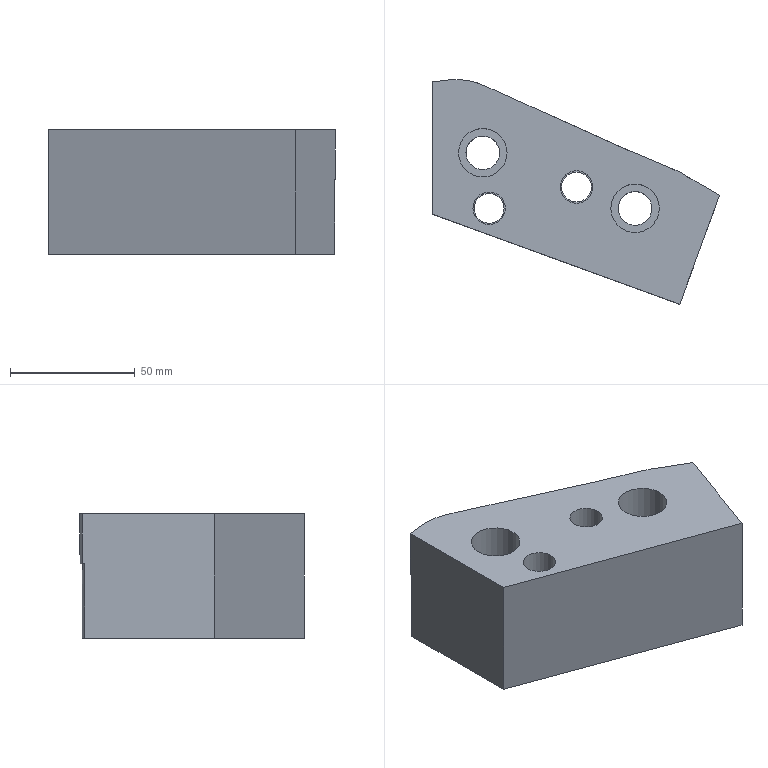Part | NX | features solid 2 | 1 solid | 23 faces | box 115.07 x 90.062 x 50 mm | volume 264486 mm3 | plane 13 | cylinder 8 | spline 2 | commonest cylinder face diameters 12 x2 13 x2 13.5 x2 19.5 x2
STEP:
#1=CARTESIAN_POINT('',(409.722,86.331,-20.));
#2=VERTEX_POINT('',#1);
#3=CARTESIAN_POINT('',(396.631,93.889,-20.));
#4=VERTEX_POINT('',#3);
#5=CARTESIAN_POINT('',(49.747,294.163,-20.));
#6=DIRECTION('',(0.866,-0.5,0.));
#7=VECTOR('',#6,1000.);
#8=LINE('',#5,#7);
#9=EDGE_CURVE('',#2,#4,#8,.F.);
#10=ORIENTED_EDGE('',*,*,#9,.T.);
#11=CARTESIAN_POINT('',(295.,131.707,-20.));
#12=VERTEX_POINT('',#11);
#13=CARTESIAN_POINT('',(396.631,93.889,-20.));
#14=CARTESIAN_POINT('',(395.875,94.532,-20.));
#15=CARTESIAN_POINT('',(393.947,95.547,-20.));
#16=CARTESIAN_POINT('',(390.75,97.031,-20.));
#17=CARTESIAN_POINT('',(387.669,98.355,-20.));
#18=CARTESIAN_POINT('',(383.326,99.967,-20.));
#19=CARTESIAN_POINT('',(377.97,102.219,-20.));
#20=CARTESIAN_POINT('',(369.545,105.997,-20.));
#21=CARTESIAN_POINT('',(359.032,110.723,-20.));
#22=CARTESIAN_POINT('',(346.404,116.383,-20.));
#23=CARTESIAN_POINT('',(335.885,121.105,-20.));
#24=CARTESIAN_POINT('',(327.471,124.89,-20.));
#25=CARTESIAN_POINT('',(322.219,127.254,-20.));
#26=CARTESIAN_POINT('',(318.003,129.177,-20.));
#27=CARTESIAN_POINT('',(314.891,130.622,-20.));
#28=CARTESIAN_POINT('',(311.756,131.732,-20.));
#29=CARTESIAN_POINT('',(307.396,132.672,-20.));
#30=CARTESIAN_POINT('',(301.819,132.728,-20.));
#31=CARTESIAN_POINT('',(297.285,132.035,-20.));
#32=CARTESIAN_POINT('',(295.,131.707,-20.));
#33=B_SPLINE_CURVE_WITH_KNOTS('',3,(#13,#14,#15,#16,#17,#18,#19,#20,#21,#22,#23,#24,#25,#26,#27,#28,#29,#30,#31,#32),.UNSPECIFIED.,.F.,.F.,(4,1,1,1,1,1,1,1,1,1,1,1,1,1,1,1,1,4),(0.7727,0.7742,0.7756,0.7771,0.7786,0.7816,0.7845,0.7904,0.7964,0.8023,0.8052,0.8082,0.8097,0.8112,0.8126,0.8141,0.8171,0.82),.UNSPECIFIED.);
#34=EDGE_CURVE('',#4,#12,#33,.T.);
#35=ORIENTED_EDGE('',*,*,#34,.T.);
#36=CARTESIAN_POINT('',(295.,132.717,-20.));
#37=VERTEX_POINT('',#36);
#38=CARTESIAN_POINT('',(295.,32.206,-20.));
#39=DIRECTION('',(0.,1.,0.));
#40=VECTOR('',#39,1000.);
#41=LINE('',#38,#40);
#42=EDGE_CURVE('',#12,#37,#41,.T.);
#43=ORIENTED_EDGE('',*,*,#42,.T.);
#44=CARTESIAN_POINT('',(397.207,94.712,-20.));
#45=VERTEX_POINT('',#44);
#46=CARTESIAN_POINT('',(-190.231,-121.49,-20.));
#47=CARTESIAN_POINT('',(-188.654,-121.152,-20.));
#48=CARTESIAN_POINT('',(-185.47,-120.627,-20.));
#49=CARTESIAN_POINT('',(-180.656,-120.141,-20.));
#50=CARTESIAN_POINT('',(-175.882,-119.326,-20.));
#51=CARTESIAN_POINT('',(-169.679,-117.528,-20.));
#52=CARTESIAN_POINT('',(-162.185,-114.539,-20.));
#53=CARTESIAN_POINT('',(-153.086,-111.254,-20.));
#54=CARTESIAN_POINT('',(-144.031,-107.845,-20.));
#55=CARTESIAN_POINT('',(-136.465,-105.061,-20.));
#56=CARTESIAN_POINT('',(-130.418,-102.814,-20.));
#57=CARTESIAN_POINT('',(-125.812,-101.329,-20.));
#58=CARTESIAN_POINT('',(-121.306,-99.566,-20.));
#59=CARTESIAN_POINT('',(-116.876,-97.626,-20.));
#60=CARTESIAN_POINT('',(-112.335,-95.923,-20.));
#61=CARTESIAN_POINT('',(-107.564,-95.05,-20.));
#62=CARTESIAN_POINT('',(-102.756,-94.525,-20.));
#63=CARTESIAN_POINT('',(-96.349,-93.771,-20.));
#64=CARTESIAN_POINT('',(-89.902,-93.468,-20.));
#65=CARTESIAN_POINT('',(-83.452,-93.448,-20.));
#66=CARTESIAN_POINT('',(-77.002,-93.469,-20.));
#67=CARTESIAN_POINT('',(-68.939,-93.411,-20.));
#68=CARTESIAN_POINT('',(-56.04,-93.3,-20.));
#69=CARTESIAN_POINT('',(-33.465,-93.184,-20.));
#70=CARTESIAN_POINT('',(-7.666,-93.074,-20.));
#71=CARTESIAN_POINT('',(14.907,-92.653,-20.));
#72=CARTESIAN_POINT('',(27.794,-92.068,-20.));
#73=CARTESIAN_POINT('',(40.668,-91.245,-20.));
#74=CARTESIAN_POINT('',(51.917,-90.291,-20.));
#75=CARTESIAN_POINT('',(61.528,-89.174,-20.));
#76=CARTESIAN_POINT('',(67.939,-88.466,-20.));
#77=CARTESIAN_POINT('',(79.125,-86.95,-20.));
#78=CARTESIAN_POINT('',(95.161,-85.253,-20.));
#79=CARTESIAN_POINT('',(114.404,-83.21,-20.));
#80=CARTESIAN_POINT('',(133.568,-80.524,-20.));
#81=CARTESIAN_POINT('',(152.734,-77.861,-20.));
#82=CARTESIAN_POINT('',(171.916,-75.326,-20.));
#83=CARTESIAN_POINT('',(191.055,-72.413,-20.));
#84=CARTESIAN_POINT('',(207.17,-71.468,-20.));
#85=CARTESIAN_POINT('',(219.951,-69.697,-20.));
#86=CARTESIAN_POINT('',(232.724,-67.899,-20.));
#87=CARTESIAN_POINT('',(248.708,-65.766,-20.));
#88=CARTESIAN_POINT('',(267.87,-63.074,-20.));
#89=CARTESIAN_POINT('',(287.038,-60.44,-20.));
#90=CARTESIAN_POINT('',(301.448,-58.682,-20.));
#91=CARTESIAN_POINT('',(310.976,-56.987,-20.));
#92=CARTESIAN_POINT('',(314.916,-56.135,-20.));
#93=CARTESIAN_POINT('',(318.052,-55.382,-20.));
#94=CARTESIAN_POINT('',(320.39,-54.76,-20.));
#95=CARTESIAN_POINT('',(322.686,-53.981,-20.));
#96=CARTESIAN_POINT('',(325.595,-52.578,-20.));
#97=CARTESIAN_POINT('',(328.769,-50.098,-20.));
#98=CARTESIAN_POINT('',(332.247,-46.69,-20.));
#99=CARTESIAN_POINT('',(335.795,-43.406,-20.));
#100=CARTESIAN_POINT('',(343.661,-37.758,-20.));
#101=CARTESIAN_POINT('',(355.164,-28.914,-20.));
#102=CARTESIAN_POINT('',(370.422,-17.018,-20.));
#103=CARTESIAN_POINT('',(383.264,-7.249,-20.));
#104=CARTESIAN_POINT('',(392.416,-0.6713,-20.));
#105=CARTESIAN_POINT('',(396.953,2.733,-20.));
#106=CARTESIAN_POINT('',(398.886,5.372,-20.));
#107=CARTESIAN_POINT('',(399.725,7.654,-20.));
#108=CARTESIAN_POINT('',(399.76,10.078,-20.));
#109=CARTESIAN_POINT('',(399.483,13.317,-20.));
#110=CARTESIAN_POINT('',(399.712,17.34,-20.));
#111=CARTESIAN_POINT('',(399.612,22.179,-20.));
#112=CARTESIAN_POINT('',(399.633,31.854,-20.));
#113=CARTESIAN_POINT('',(399.593,46.366,-20.));
#114=CARTESIAN_POINT('',(399.637,62.491,-20.));
#115=CARTESIAN_POINT('',(399.588,73.779,-20.));
#116=CARTESIAN_POINT('',(399.652,79.422,-20.));
#117=CARTESIAN_POINT('',(399.59,82.647,-20.));
#118=CARTESIAN_POINT('',(399.564,85.065,-20.));
#119=CARTESIAN_POINT('',(399.725,87.486,-20.));
#120=CARTESIAN_POINT('',(399.756,89.902,-20.));
#121=CARTESIAN_POINT('',(399.247,92.301,-20.));
#122=CARTESIAN_POINT('',(397.362,95.008,-20.));
#123=CARTESIAN_POINT('',(393.635,96.774,-20.));
#124=CARTESIAN_POINT('',(389.279,98.826,-20.));
#125=CARTESIAN_POINT('',(384.732,100.498,-20.));
#126=CARTESIAN_POINT('',(378.765,102.95,-20.));
#127=CARTESIAN_POINT('',(362.589,110.229,-20.));
#128=CARTESIAN_POINT('',(344.928,118.135,-20.));
#129=CARTESIAN_POINT('',(327.281,126.072,-20.));
#130=CARTESIAN_POINT('',(319.932,129.381,-20.));
#131=CARTESIAN_POINT('',(314.075,132.102,-20.));
#132=CARTESIAN_POINT('',(309.387,133.376,-20.));
#133=CARTESIAN_POINT('',(304.547,133.785,-20.));
#134=CARTESIAN_POINT('',(299.716,133.401,-20.));
#135=CARTESIAN_POINT('',(294.929,132.704,-20.));
#136=CARTESIAN_POINT('',(288.543,131.8,-20.));
#137=CARTESIAN_POINT('',(277.364,130.241,-20.));
#138=CARTESIAN_POINT('',(242.2,125.552,-20.));
#139=CARTESIAN_POINT('',(184.637,118.048,-20.));
#140=CARTESIAN_POINT('',(120.701,109.541,-20.));
#141=CARTESIAN_POINT('',(69.531,102.902,-20.));
#142=CARTESIAN_POINT('',(40.777,98.94,-20.));
#143=CARTESIAN_POINT('',(21.566,96.615,-20.));
#144=CARTESIAN_POINT('',(8.743,95.212,-20.));
#145=CARTESIAN_POINT('',(-7.301,93.575,-20.));
#146=CARTESIAN_POINT('',(-26.625,92.505,-20.));
#147=CARTESIAN_POINT('',(-45.971,92.017,-20.));
#148=CARTESIAN_POINT('',(-62.09,91.675,-20.));
#149=CARTESIAN_POINT('',(-74.987,91.256,-20.));
#150=CARTESIAN_POINT('',(-84.664,91.165,-20.));
#151=CARTESIAN_POINT('',(-94.319,91.781,-20.));
#152=CARTESIAN_POINT('',(-103.929,92.966,-20.));
#153=CARTESIAN_POINT('',(-113.495,94.403,-20.));
#154=CARTESIAN_POINT('',(-119.856,95.492,-20.));
#155=CARTESIAN_POINT('',(-122.997,96.222,-20.));
#156=B_SPLINE_CURVE_WITH_KNOTS('',3,(#46,#47,#48,#49,#50,#51,#52,#53,#54,#55,#56,#57,#58,#59,#60,#61,#62,#63,#64,#65,#66,#67,#68,#69,#70,#71,#72,#73,#74,#75,#76,#77,#78,#79,#80,#81,#82,#83,#84,#85,#86,#87,#88,#89,#90,#91,#92,#93,#94,#95,#96,#97,#98,#99,#100,#101,#102,#103,#104,#105,#106,#107,#108,#109,#110,#111,#112,#113,#114,#115,#116,#117,#118,#119,#120,#121,#122,#123,#124,#125,#126,#127,#128,#129,#130,#131,#132,#133,#134,#135,#136,#137,#138,#139,#140,#141,#142,#143,#144,#145,#146,#147,#148,#149,#150,#151,#152,#153,#154,#155),.UNSPECIFIED.,.F.,.F.,(4,1,1,1,1,1,1,1,1,1,1,1,1,1,1,1,1,1,1,1,1,1,1,1,1,1,1,1,1,1,1,1,1,1,1,1,1,1,1,1,1,1,1,1,1,1,1,1,1,1,1,1,1,1,1,1,1,1,1,1,1,1,1,1,1,1,1,1,1,1,1,1,1,1,1,1,1,1,1,1,1,1,1,1,1,1,1,1,1,1,1,1,1,1,1,1,1,1,1,1,1,1,1,1,1,1,1,4),(0.4704,0.4724,0.4745,0.4766,0.4786,0.4828,0.4869,0.491,0.4952,0.4972,0.4993,0.5014,0.5035,0.5055,0.5076,0.5097,0.5117,0.5159,0.5179,0.52,0.5241,0.5283,0.5366,0.5531,0.5614,0.5655,0.5697,0.5779,0.58,0.5821,0.5862,0.5945,0.6028,0.611,0.6193,0.6276,0.6359,0.6441,0.6483,0.6524,0.6607,0.669,0.6772,0.6855,0.6876,0.6897,0.6907,0.6917,0.6928,0.6938,0.6959,0.6979,0.7,0.7021,0.7103,0.7186,0.7269,0.731,0.7331,0.7341,0.7352,0.7362,0.7372,0.7393,0.7414,0.7435,0.7517,0.76,0.7641,0.7662,0.7672,0.7683,0.7693,0.7703,0.7714,0.7724,0.7745,0.7766,0.7786,0.7807,0.7848,0.8014,0.8055,0.8097,0.8117,0.8138,0.8159,0.8179,0.82,0.8221,0.8262,0.8345,0.8676,0.9007,0.9172,0.9338,0.9379,0.9421,0.9503,0.9586,0.9669,0.9752,0.9793,0.9834,0.9876,0.9917,0.9959,1.),.UNSPECIFIED.);
#157=EDGE_CURVE('',#45,#37,#156,.T.);
#158=ORIENTED_EDGE('',*,*,#157,.F.);
#159=CARTESIAN_POINT('',(410.07,87.285,-20.));
#160=VERTEX_POINT('',#159);
#161=CARTESIAN_POINT('',(409.267,87.749,-20.));
#162=DIRECTION('',(-0.866,0.5,0.));
#163=VECTOR('',#162,1000.);
#164=LINE('',#161,#163);
#165=EDGE_CURVE('',#160,#45,#164,.T.);
#166=ORIENTED_EDGE('',*,*,#165,.F.);
#167=CARTESIAN_POINT('',(395.302,46.71,-20.));
#168=DIRECTION('',(-0.342,-0.9397,0.));
#169=VECTOR('',#168,1000.);
#170=LINE('',#167,#169);
#171=EDGE_CURVE('',#160,#2,#170,.T.);
#172=ORIENTED_EDGE('',*,*,#171,.T.);
#173=EDGE_LOOP('',(#10,#35,#43,#158,#166,#172));
#174=FACE_BOUND('',#173,.T.);
#175=CARTESIAN_POINT('',(-190.231,-121.49,-20.));
#176=DIRECTION('',(0.,0.,1.));
#177=DIRECTION('',(1.,0.,0.));
#178=AXIS2_PLACEMENT_3D('',#175,#176,#177);
#179=PLANE('',#178);
#180=ADVANCED_FACE('',(#174),#179,.F.);
#181=CARTESIAN_POINT('',(396.631,93.889,-50.));
#182=VERTEX_POINT('',#181);
#183=CARTESIAN_POINT('',(396.631,93.889,-35.));
#184=DIRECTION('',(0.,0.,-1.));
#185=VECTOR('',#184,1000.);
#186=LINE('',#183,#185);
#187=EDGE_CURVE('',#182,#4,#186,.F.);
#188=ORIENTED_EDGE('',*,*,#187,.F.);
#189=CARTESIAN_POINT('',(295.,131.707,-50.));
#190=VERTEX_POINT('',#189);
#191=CARTESIAN_POINT('',(295.,131.707,-50.));
#192=CARTESIAN_POINT('',(297.276,132.034,-50.));
#193=CARTESIAN_POINT('',(301.806,132.738,-50.));
#194=CARTESIAN_POINT('',(307.62,132.66,-50.));
#195=CARTESIAN_POINT('',(312.106,131.636,-50.));
#196=CARTESIAN_POINT('',(315.302,130.443,-50.));
#197=CARTESIAN_POINT('',(318.413,128.985,-50.));
#198=CARTESIAN_POINT('',(322.577,127.094,-50.));
#199=CARTESIAN_POINT('',(327.792,124.745,-50.));
#200=CARTESIAN_POINT('',(336.136,120.993,-50.));
#201=CARTESIAN_POINT('',(346.569,116.309,-50.));
#202=CARTESIAN_POINT('',(359.092,110.696,-50.));
#203=CARTESIAN_POINT('',(369.523,106.007,-50.));
#204=CARTESIAN_POINT('',(377.871,102.264,-50.));
#205=CARTESIAN_POINT('',(383.139,100.041,-50.));
#206=CARTESIAN_POINT('',(387.428,98.446,-50.));
#207=CARTESIAN_POINT('',(390.592,97.111,-50.));
#208=CARTESIAN_POINT('',(393.681,95.654,-50.));
#209=CARTESIAN_POINT('',(395.755,94.633,-50.));
#210=CARTESIAN_POINT('',(396.631,93.889,-50.));
#211=B_SPLINE_CURVE_WITH_KNOTS('',3,(#191,#192,#193,#194,#195,#196,#197,#198,#199,#200,#201,#202,#203,#204,#205,#206,#207,#208,#209,#210),.UNSPECIFIED.,.F.,.F.,(4,1,1,1,1,1,1,1,1,1,1,1,1,1,1,1,1,4),(0.,0.006873,0.01375,0.01718,0.02062,0.02406,0.02749,0.03437,0.04124,0.05499,0.06873,0.08248,0.08935,0.09623,0.09966,0.1031,0.1065,0.11),.UNSPECIFIED.);
#212=EDGE_CURVE('',#190,#182,#211,.T.);
#213=ORIENTED_EDGE('',*,*,#212,.F.);
#214=CARTESIAN_POINT('',(295.,131.707,-60.));
#215=DIRECTION('',(0.,0.,-1.));
#216=VECTOR('',#215,1000.);
#217=LINE('',#214,#216);
#218=EDGE_CURVE('',#190,#12,#217,.F.);
#219=ORIENTED_EDGE('',*,*,#218,.T.);
#220=ORIENTED_EDGE('',*,*,#34,.F.);
#221=EDGE_LOOP('',(#188,#213,#219,#220));
#222=FACE_BOUND('',#221,.T.);
#223=CARTESIAN_POINT('',(396.631,93.889,-20.));
#224=CARTESIAN_POINT('',(396.631,93.889,-50.));
#225=CARTESIAN_POINT('',(395.875,94.532,-20.));
#226=CARTESIAN_POINT('',(395.875,94.532,-50.));
#227=CARTESIAN_POINT('',(393.947,95.547,-20.));
#228=CARTESIAN_POINT('',(393.947,95.547,-50.));
#229=CARTESIAN_POINT('',(390.75,97.031,-20.));
#230=CARTESIAN_POINT('',(390.75,97.031,-50.));
#231=CARTESIAN_POINT('',(387.669,98.355,-20.));
#232=CARTESIAN_POINT('',(387.669,98.355,-50.));
#233=CARTESIAN_POINT('',(383.326,99.967,-20.));
#234=CARTESIAN_POINT('',(383.326,99.967,-50.));
#235=CARTESIAN_POINT('',(377.97,102.219,-20.));
#236=CARTESIAN_POINT('',(377.97,102.219,-50.));
#237=CARTESIAN_POINT('',(369.545,105.997,-20.));
#238=CARTESIAN_POINT('',(369.545,105.997,-50.));
#239=CARTESIAN_POINT('',(359.032,110.723,-20.));
#240=CARTESIAN_POINT('',(359.032,110.723,-50.));
#241=CARTESIAN_POINT('',(346.404,116.383,-20.));
#242=CARTESIAN_POINT('',(346.404,116.383,-50.));
#243=CARTESIAN_POINT('',(335.885,121.105,-20.));
#244=CARTESIAN_POINT('',(335.885,121.105,-50.));
#245=CARTESIAN_POINT('',(327.471,124.89,-20.));
#246=CARTESIAN_POINT('',(327.471,124.89,-50.));
#247=CARTESIAN_POINT('',(322.219,127.254,-20.));
#248=CARTESIAN_POINT('',(322.219,127.254,-50.));
#249=CARTESIAN_POINT('',(318.003,129.177,-20.));
#250=CARTESIAN_POINT('',(318.003,129.177,-50.));
#251=CARTESIAN_POINT('',(314.891,130.622,-20.));
#252=CARTESIAN_POINT('',(314.891,130.622,-50.));
#253=CARTESIAN_POINT('',(311.756,131.732,-20.));
#254=CARTESIAN_POINT('',(311.756,131.732,-50.));
#255=CARTESIAN_POINT('',(307.396,132.672,-20.));
#256=CARTESIAN_POINT('',(307.396,132.672,-50.));
#257=CARTESIAN_POINT('',(301.819,132.728,-20.));
#258=CARTESIAN_POINT('',(301.819,132.728,-50.));
#259=CARTESIAN_POINT('',(297.285,132.035,-20.));
#260=CARTESIAN_POINT('',(297.285,132.035,-50.));
#261=CARTESIAN_POINT('',(295.,131.707,-20.));
#262=CARTESIAN_POINT('',(295.,131.707,-50.));
#263=B_SPLINE_SURFACE_WITH_KNOTS('',3,1,((#223,#224),(#225,#226),(#227,#228),(#229,#230),(#231,#232),(#233,#234),(#235,#236),(#237,#238),(#239,#240),(#241,#242),(#243,#244),(#245,#246),(#247,#248),(#249,#250),(#251,#252),(#253,#254),(#255,#256),(#257,#258),(#259,#260),(#261,#262)),.SURF_OF_LINEAR_EXTRUSION.,.F.,.F.,.F.,(4,1,1,1,1,1,1,1,1,1,1,1,1,1,1,1,1,4),(2,2),(0.7727,0.7742,0.7756,0.7771,0.7786,0.7816,0.7845,0.7904,0.7964,0.8023,0.8052,0.8082,0.8097,0.8112,0.8126,0.8141,0.8171,0.82),(0.,1.),.UNSPECIFIED.);
#264=ADVANCED_FACE('',(#222),#263,.F.);
#265=CARTESIAN_POINT('',(409.722,86.331,-50.));
#266=VERTEX_POINT('',#265);
#267=CARTESIAN_POINT('',(403.304,68.696,-50.));
#268=VERTEX_POINT('',#267);
#269=CARTESIAN_POINT('',(395.302,46.71,-50.));
#270=DIRECTION('',(-0.342,-0.9397,0.));
#271=VECTOR('',#270,1000.);
#272=LINE('',#269,#271);
#273=EDGE_CURVE('',#266,#268,#272,.T.);
#274=ORIENTED_EDGE('',*,*,#273,.F.);
#275=CARTESIAN_POINT('',(409.722,86.331,0.));
#276=DIRECTION('',(0.,0.,-1.));
#277=VECTOR('',#276,1000.);
#278=LINE('',#275,#277);
#279=EDGE_CURVE('',#2,#266,#278,.T.);
#280=ORIENTED_EDGE('',*,*,#279,.F.);
#281=ORIENTED_EDGE('',*,*,#171,.F.);
#282=CARTESIAN_POINT('',(410.07,87.285,0.));
#283=VERTEX_POINT('',#282);
#284=CARTESIAN_POINT('',(410.07,87.285,0.));
#285=DIRECTION('',(0.,0.,-1.));
#286=VECTOR('',#285,1000.);
#287=LINE('',#284,#286);
#288=EDGE_CURVE('',#160,#283,#287,.F.);
#289=ORIENTED_EDGE('',*,*,#288,.T.);
#290=CARTESIAN_POINT('',(394.166,43.591,0.));
#291=VERTEX_POINT('',#290);
#292=CARTESIAN_POINT('',(207.674,-468.792,0.));
#293=DIRECTION('',(-0.342,-0.9397,0.));
#294=VECTOR('',#293,1000.);
#295=LINE('',#292,#294);
#296=EDGE_CURVE('',#283,#291,#295,.T.);
#297=ORIENTED_EDGE('',*,*,#296,.T.);
#298=CARTESIAN_POINT('',(394.166,43.591,-50.));
#299=VERTEX_POINT('',#298);
#300=CARTESIAN_POINT('',(394.166,43.591,0.));
#301=DIRECTION('',(0.,0.,-1.));
#302=VECTOR('',#301,1000.);
#303=LINE('',#300,#302);
#304=EDGE_CURVE('',#291,#299,#303,.T.);
#305=ORIENTED_EDGE('',*,*,#304,.T.);
#306=CARTESIAN_POINT('',(296.724,-224.13,-50.));
#307=DIRECTION('',(0.342,0.9397,0.));
#308=VECTOR('',#307,1000.);
#309=LINE('',#306,#308);
#310=EDGE_CURVE('',#268,#299,#309,.F.);
#311=ORIENTED_EDGE('',*,*,#310,.F.);
#312=CARTESIAN_POINT('',(403.304,68.696,-20.));
#313=VERTEX_POINT('',#312);
#314=CARTESIAN_POINT('',(403.304,68.696,0.));
#315=DIRECTION('',(0.,0.,1.));
#316=VECTOR('',#315,1000.);
#317=LINE('',#314,#316);
#318=EDGE_CURVE('',#313,#268,#317,.F.);
#319=ORIENTED_EDGE('',*,*,#318,.F.);
#320=ORIENTED_EDGE('',*,*,#318,.T.);
#321=EDGE_LOOP('',(#274,#280,#281,#289,#297,#305,#311,#319,#320));
#322=FACE_BOUND('',#321,.T.);
#323=CARTESIAN_POINT('',(395.302,46.71,0.));
#324=DIRECTION('',(0.9397,-0.342,0.));
#325=DIRECTION('',(0.342,0.9397,0.));
#326=AXIS2_PLACEMENT_3D('',#323,#324,#325);
#327=PLANE('',#326);
#328=ADVANCED_FACE('',(#322),#327,.T.);
#329=CARTESIAN_POINT('',(346.244,90.593,0.));
#330=VERTEX_POINT('',#329);
#331=CARTESIAN_POINT('',(352.744,90.593,0.));
#332=DIRECTION('',(0.,0.,-1.));
#333=DIRECTION('',(-1.,0.,0.));
#334=AXIS2_PLACEMENT_3D('',#331,#332,#333);
#335=CIRCLE('',#334,6.5);
#336=EDGE_CURVE('',#330,#330,#335,.T.);
#337=ORIENTED_EDGE('',*,*,#336,.T.);
#338=EDGE_LOOP('',(#337));
#339=FACE_BOUND('',#338,.T.);
#340=CARTESIAN_POINT('',(311.213,82.06,0.));
#341=VERTEX_POINT('',#340);
#342=CARTESIAN_POINT('',(317.713,82.06,0.));
#343=DIRECTION('',(0.,0.,-1.));
#344=DIRECTION('',(-1.,0.,0.));
#345=AXIS2_PLACEMENT_3D('',#342,#343,#344);
#346=CIRCLE('',#345,6.5);
#347=EDGE_CURVE('',#341,#341,#346,.T.);
#348=ORIENTED_EDGE('',*,*,#347,.T.);
#349=EDGE_LOOP('',(#348));
#350=FACE_BOUND('',#349,.T.);
#351=CARTESIAN_POINT('',(366.486,82.043,0.));
#352=VERTEX_POINT('',#351);
#353=CARTESIAN_POINT('',(376.236,82.043,0.));
#354=DIRECTION('',(0.,0.,-1.));
#355=DIRECTION('',(-1.,0.,0.));
#356=AXIS2_PLACEMENT_3D('',#353,#354,#355);
#357=CIRCLE('',#356,9.75);
#358=EDGE_CURVE('',#352,#352,#357,.T.);
#359=ORIENTED_EDGE('',*,*,#358,.T.);
#360=EDGE_LOOP('',(#359));
#361=FACE_BOUND('',#360,.T.);
#362=CARTESIAN_POINT('',(305.406,104.274,0.));
#363=VERTEX_POINT('',#362);
#364=CARTESIAN_POINT('',(315.156,104.274,0.));
#365=DIRECTION('',(0.,0.,-1.));
#366=DIRECTION('',(-1.,0.,0.));
#367=AXIS2_PLACEMENT_3D('',#364,#365,#366);
#368=CIRCLE('',#367,9.75);
#369=EDGE_CURVE('',#363,#363,#368,.T.);
#370=ORIENTED_EDGE('',*,*,#369,.T.);
#371=EDGE_LOOP('',(#370));
#372=FACE_BOUND('',#371,.T.);
#373=CARTESIAN_POINT('',(295.,79.685,0.));
#374=VERTEX_POINT('',#373);
#375=CARTESIAN_POINT('',(-283.889,290.383,0.));
#376=DIRECTION('',(-0.9397,0.342,0.));
#377=VECTOR('',#376,1000.);
#378=LINE('',#375,#377);
#379=EDGE_CURVE('',#291,#374,#378,.T.);
#380=ORIENTED_EDGE('',*,*,#379,.F.);
#381=ORIENTED_EDGE('',*,*,#296,.F.);
#382=CARTESIAN_POINT('',(397.411,94.594,0.));
#383=VERTEX_POINT('',#382);
#384=CARTESIAN_POINT('',(409.267,87.749,0.));
#385=DIRECTION('',(0.866,-0.5,0.));
#386=VECTOR('',#385,1000.);
#387=LINE('',#384,#386);
#388=EDGE_CURVE('',#283,#383,#387,.F.);
#389=ORIENTED_EDGE('',*,*,#388,.T.);
#390=CARTESIAN_POINT('',(397.389,94.556,0.));
#391=VERTEX_POINT('',#390);
#392=CARTESIAN_POINT('',(43.373,-518.616,0.));
#393=DIRECTION('',(0.5,0.866,0.));
#394=VECTOR('',#393,1000.);
#395=LINE('',#392,#394);
#396=EDGE_CURVE('',#391,#383,#395,.T.);
#397=ORIENTED_EDGE('',*,*,#396,.F.);
#398=CARTESIAN_POINT('',(295.,132.717,0.));
#399=VERTEX_POINT('',#398);
#400=CARTESIAN_POINT('',(397.389,94.556,0.));
#401=CARTESIAN_POINT('',(396.507,95.335,0.));
#402=CARTESIAN_POINT('',(394.465,96.407,0.));
#403=CARTESIAN_POINT('',(391.331,97.864,0.));
#404=CARTESIAN_POINT('',(388.159,99.24,0.));
#405=CARTESIAN_POINT('',(383.835,100.843,0.));
#406=CARTESIAN_POINT('',(378.522,103.069,0.));
#407=CARTESIAN_POINT('',(370.109,106.839,0.));
#408=CARTESIAN_POINT('',(359.6,111.565,0.));
#409=CARTESIAN_POINT('',(346.981,117.22,0.));
#410=CARTESIAN_POINT('',(336.469,121.94,0.));
#411=CARTESIAN_POINT('',(328.061,125.721,0.));
#412=CARTESIAN_POINT('',(322.807,128.087,0.));
#413=CARTESIAN_POINT('',(318.613,129.995,0.));
#414=CARTESIAN_POINT('',(314.432,131.951,0.));
#415=CARTESIAN_POINT('',(308.984,133.624,0.));
#416=CARTESIAN_POINT('',(301.881,133.753,0.));
#417=CARTESIAN_POINT('',(297.3,133.048,0.));
#418=CARTESIAN_POINT('',(295.,132.717,0.));
#419=B_SPLINE_CURVE_WITH_KNOTS('',3,(#400,#401,#402,#403,#404,#405,#406,#407,#408,#409,#410,#411,#412,#413,#414,#415,#416,#417,#418),.UNSPECIFIED.,.F.,.F.,(4,1,1,1,1,1,1,1,1,1,1,1,1,1,1,1,4),(0.1889,0.1924,0.1959,0.1993,0.2028,0.2097,0.2167,0.2305,0.2444,0.2583,0.2652,0.2721,0.2756,0.2791,0.286,0.293,0.2999),.UNSPECIFIED.);
#420=EDGE_CURVE('',#399,#391,#419,.F.);
#421=ORIENTED_EDGE('',*,*,#420,.F.);
#422=CARTESIAN_POINT('',(295.,-222.,0.));
#423=DIRECTION('',(0.,1.,0.));
#424=VECTOR('',#423,1000.);
#425=LINE('',#422,#424);
#426=EDGE_CURVE('',#374,#399,#425,.T.);
#427=ORIENTED_EDGE('',*,*,#426,.F.);
#428=EDGE_LOOP('',(#380,#381,#389,#397,#421,#427));
#429=FACE_BOUND('',#428,.T.);
#430=CARTESIAN_POINT('',(-470.381,-222.,0.));
#431=DIRECTION('',(0.,0.,-1.));
#432=DIRECTION('',(-1.,0.,0.));
#433=AXIS2_PLACEMENT_3D('',#430,#431,#432);
#434=PLANE('',#433);
#435=ADVANCED_FACE('',(#339,#350,#361,#372,#429),#434,.F.);
#436=ORIENTED_EDGE('',*,*,#212,.T.);
#437=CARTESIAN_POINT('',(-186.99,430.843,-50.));
#438=DIRECTION('',(0.866,-0.5,0.));
#439=VECTOR('',#438,1000.);
#440=LINE('',#437,#439);
#441=EDGE_CURVE('',#266,#182,#440,.F.);
#442=ORIENTED_EDGE('',*,*,#441,.F.);
#443=ORIENTED_EDGE('',*,*,#273,.T.);
#444=ORIENTED_EDGE('',*,*,#310,.T.);
#445=CARTESIAN_POINT('',(295.,79.685,-50.));
#446=VERTEX_POINT('',#445);
#447=CARTESIAN_POINT('',(-318.035,302.812,-50.));
#448=DIRECTION('',(0.9397,-0.342,0.));
#449=VECTOR('',#448,1000.);
#450=LINE('',#447,#449);
#451=EDGE_CURVE('',#446,#299,#450,.T.);
#452=ORIENTED_EDGE('',*,*,#451,.F.);
#453=CARTESIAN_POINT('',(295.,35.09,-50.));
#454=DIRECTION('',(0.,-1.,0.));
#455=VECTOR('',#454,1000.);
#456=LINE('',#453,#455);
#457=EDGE_CURVE('',#190,#446,#456,.T.);
#458=ORIENTED_EDGE('',*,*,#457,.F.);
#459=EDGE_LOOP('',(#436,#442,#443,#444,#452,#458));
#460=FACE_BOUND('',#459,.T.);
#461=CARTESIAN_POINT('',(321.906,104.274,-50.));
#462=VERTEX_POINT('',#461);
#463=CARTESIAN_POINT('',(315.156,104.274,-50.));
#464=DIRECTION('',(0.,0.,1.));
#465=DIRECTION('',(1.,0.,0.));
#466=AXIS2_PLACEMENT_3D('',#463,#464,#465);
#467=CIRCLE('',#466,6.75);
#468=EDGE_CURVE('',#462,#462,#467,.T.);
#469=ORIENTED_EDGE('',*,*,#468,.T.);
#470=EDGE_LOOP('',(#469));
#471=FACE_BOUND('',#470,.T.);
#472=CARTESIAN_POINT('',(382.986,82.043,-50.));
#473=VERTEX_POINT('',#472);
#474=CARTESIAN_POINT('',(376.236,82.043,-50.));
#475=DIRECTION('',(0.,0.,1.));
#476=DIRECTION('',(1.,0.,0.));
#477=AXIS2_PLACEMENT_3D('',#474,#475,#476);
#478=CIRCLE('',#477,6.75);
#479=EDGE_CURVE('',#473,#473,#478,.T.);
#480=ORIENTED_EDGE('',*,*,#479,.T.);
#481=EDGE_LOOP('',(#480));
#482=FACE_BOUND('',#481,.T.);
#483=CARTESIAN_POINT('',(323.713,82.06,-50.));
#484=VERTEX_POINT('',#483);
#485=CARTESIAN_POINT('',(317.713,82.06,-50.));
#486=DIRECTION('',(0.,0.,1.));
#487=DIRECTION('',(1.,0.,0.));
#488=AXIS2_PLACEMENT_3D('',#485,#486,#487);
#489=CIRCLE('',#488,6.);
#490=EDGE_CURVE('',#484,#484,#489,.T.);
#491=ORIENTED_EDGE('',*,*,#490,.T.);
#492=EDGE_LOOP('',(#491));
#493=FACE_BOUND('',#492,.T.);
#494=CARTESIAN_POINT('',(358.744,90.593,-50.));
#495=VERTEX_POINT('',#494);
#496=CARTESIAN_POINT('',(352.744,90.593,-50.));
#497=DIRECTION('',(0.,0.,1.));
#498=DIRECTION('',(1.,0.,0.));
#499=AXIS2_PLACEMENT_3D('',#496,#497,#498);
#500=CIRCLE('',#499,6.);
#501=EDGE_CURVE('',#495,#495,#500,.T.);
#502=ORIENTED_EDGE('',*,*,#501,.T.);
#503=EDGE_LOOP('',(#502));
#504=FACE_BOUND('',#503,.T.);
#505=CARTESIAN_POINT('',(-415.478,35.09,-50.));
#506=DIRECTION('',(0.,0.,1.));
#507=DIRECTION('',(1.,0.,0.));
#508=AXIS2_PLACEMENT_3D('',#505,#506,#507);
#509=PLANE('',#508);
#510=ADVANCED_FACE('',(#460,#471,#482,#493,#504),#509,.F.);
#511=CARTESIAN_POINT('',(397.207,94.712,-8.62));
#512=VERTEX_POINT('',#511);
#513=CARTESIAN_POINT('',(397.389,94.556,0.));
#514=CARTESIAN_POINT('',(397.329,94.609,-2.873));
#515=CARTESIAN_POINT('',(397.268,94.661,-5.747));
#516=CARTESIAN_POINT('',(397.207,94.712,-8.62));
#517=B_SPLINE_CURVE_WITH_KNOTS('',3,(#513,#514,#515,#516),.UNSPECIFIED.,.F.,.F.,(4,4),(0.,0.008624),.UNSPECIFIED.);
#518=EDGE_CURVE('',#391,#512,#517,.T.);
#519=ORIENTED_EDGE('',*,*,#518,.T.);
#520=CARTESIAN_POINT('',(397.207,94.712,-10.));
#521=DIRECTION('',(0.,0.,-1.));
#522=VECTOR('',#521,1000.);
#523=LINE('',#520,#522);
#524=EDGE_CURVE('',#512,#45,#523,.T.);
#525=ORIENTED_EDGE('',*,*,#524,.T.);
#526=ORIENTED_EDGE('',*,*,#157,.T.);
#527=CARTESIAN_POINT('',(295.,132.717,-10.));
#528=DIRECTION('',(0.,0.,-1.));
#529=VECTOR('',#528,1000.);
#530=LINE('',#527,#529);
#531=EDGE_CURVE('',#399,#37,#530,.T.);
#532=ORIENTED_EDGE('',*,*,#531,.F.);
#533=ORIENTED_EDGE('',*,*,#420,.T.);
#534=EDGE_LOOP('',(#519,#525,#526,#532,#533));
#535=FACE_BOUND('',#534,.T.);
#536=CARTESIAN_POINT('',(397.862,94.099,0.));
#537=CARTESIAN_POINT('',(397.862,94.099,-20.));
#538=CARTESIAN_POINT('',(397.072,94.939,0.));
#539=CARTESIAN_POINT('',(397.072,94.939,-20.));
#540=CARTESIAN_POINT('',(395.084,96.144,0.));
#541=CARTESIAN_POINT('',(395.084,96.144,-20.));
#542=CARTESIAN_POINT('',(391.873,97.599,0.));
#543=CARTESIAN_POINT('',(391.873,97.599,-20.));
#544=CARTESIAN_POINT('',(388.721,99.022,0.));
#545=CARTESIAN_POINT('',(388.721,99.022,-20.));
#546=CARTESIAN_POINT('',(385.453,100.238,0.));
#547=CARTESIAN_POINT('',(385.453,100.238,-20.));
#548=CARTESIAN_POINT('',(382.218,101.523,0.));
#549=CARTESIAN_POINT('',(382.218,101.523,-20.));
#550=CARTESIAN_POINT('',(377.945,103.331,0.));
#551=CARTESIAN_POINT('',(377.945,103.331,-20.));
#552=CARTESIAN_POINT('',(370.532,106.646,0.));
#553=CARTESIAN_POINT('',(370.532,106.646,-20.));
#554=CARTESIAN_POINT('',(359.953,111.407,0.));
#555=CARTESIAN_POINT('',(359.953,111.407,-20.));
#556=CARTESIAN_POINT('',(347.25,117.1,0.));
#557=CARTESIAN_POINT('',(347.25,117.1,-20.));
#558=CARTESIAN_POINT('',(336.667,121.851,0.));
#559=CARTESIAN_POINT('',(336.667,121.851,-20.));
#560=CARTESIAN_POINT('',(328.203,125.657,0.));
#561=CARTESIAN_POINT('',(328.203,125.657,-20.));
#562=CARTESIAN_POINT('',(322.917,128.038,0.));
#563=CARTESIAN_POINT('',(322.917,128.038,-20.));
#564=CARTESIAN_POINT('',(318.69,129.958,0.));
#565=CARTESIAN_POINT('',(318.69,129.958,-20.));
#566=CARTESIAN_POINT('',(314.487,131.932,0.));
#567=CARTESIAN_POINT('',(314.487,131.932,-20.));
#568=CARTESIAN_POINT('',(308.899,133.642,0.));
#569=CARTESIAN_POINT('',(308.899,133.642,-20.));
#570=CARTESIAN_POINT('',(301.889,133.747,0.));
#571=CARTESIAN_POINT('',(301.889,133.747,-20.));
#572=CARTESIAN_POINT('',(297.296,133.047,0.));
#573=CARTESIAN_POINT('',(297.296,133.047,-20.));
#574=CARTESIAN_POINT('',(295.,132.717,0.));
#575=CARTESIAN_POINT('',(295.,132.717,-20.));
#576=B_SPLINE_SURFACE_WITH_KNOTS('',3,1,((#536,#537),(#538,#539),(#540,#541),(#542,#543),(#544,#545),(#546,#547),(#548,#549),(#550,#551),(#552,#553),(#554,#555),(#556,#557),(#558,#559),(#560,#561),(#562,#563),(#564,#565),(#566,#567),(#568,#569),(#570,#571),(#572,#573),(#574,#575)),.SURF_OF_LINEAR_EXTRUSION.,.F.,.F.,.F.,(4,1,1,1,1,1,1,1,1,1,1,1,1,1,1,1,1,4),(2,2),(0.7723,0.7738,0.7753,0.7768,0.7783,0.7798,0.7813,0.7842,0.7902,0.7962,0.8021,0.8051,0.8081,0.8096,0.811,0.814,0.817,0.82),(0.,1.),.UNSPECIFIED.);
#577=ADVANCED_FACE('',(#535),#576,.F.);
#578=ORIENTED_EDGE('',*,*,#379,.T.);
#579=CARTESIAN_POINT('',(295.,79.685,-25.));
#580=DIRECTION('',(0.,0.,1.));
#581=VECTOR('',#580,1000.);
#582=LINE('',#579,#581);
#583=EDGE_CURVE('',#446,#374,#582,.T.);
#584=ORIENTED_EDGE('',*,*,#583,.F.);
#585=ORIENTED_EDGE('',*,*,#451,.T.);
#586=ORIENTED_EDGE('',*,*,#304,.F.);
#587=EDGE_LOOP('',(#578,#584,#585,#586));
#588=FACE_BOUND('',#587,.T.);
#589=CARTESIAN_POINT('',(346.123,61.078,0.));
#590=DIRECTION('',(-0.342,-0.9397,0.));
#591=DIRECTION('',(0.9397,-0.342,0.));
#592=AXIS2_PLACEMENT_3D('',#589,#590,#591);
#593=PLANE('',#592);
#594=ADVANCED_FACE('',(#588),#593,.T.);
#595=ORIENTED_EDGE('',*,*,#42,.F.);
#596=ORIENTED_EDGE('',*,*,#218,.F.);
#597=ORIENTED_EDGE('',*,*,#457,.T.);
#598=ORIENTED_EDGE('',*,*,#583,.T.);
#599=ORIENTED_EDGE('',*,*,#426,.T.);
#600=ORIENTED_EDGE('',*,*,#531,.T.);
#601=EDGE_LOOP('',(#595,#596,#597,#598,#599,#600));
#602=FACE_BOUND('',#601,.T.);
#603=CARTESIAN_POINT('',(295.,32.206,-25.));
#604=DIRECTION('',(-1.,0.,0.));
#605=DIRECTION('',(0.,0.,1.));
#606=AXIS2_PLACEMENT_3D('',#603,#604,#605);
#607=PLANE('',#606);
#608=ADVANCED_FACE('',(#602),#607,.T.);
#609=CARTESIAN_POINT('',(308.406,104.274,-15.));
#610=VERTEX_POINT('',#609);
#611=CARTESIAN_POINT('',(315.156,104.274,-15.));
#612=DIRECTION('',(0.,0.,-1.));
#613=DIRECTION('',(-1.,0.,0.));
#614=AXIS2_PLACEMENT_3D('',#611,#612,#613);
#615=CIRCLE('',#614,6.75);
#616=EDGE_CURVE('',#610,#610,#615,.T.);
#617=ORIENTED_EDGE('',*,*,#616,.F.);
#618=EDGE_LOOP('',(#617));
#619=FACE_BOUND('',#618,.T.);
#620=ORIENTED_EDGE('',*,*,#468,.F.);
#621=EDGE_LOOP('',(#620));
#622=FACE_BOUND('',#621,.T.);
#623=CARTESIAN_POINT('',(315.156,104.274,-100.));
#624=DIRECTION('',(0.,0.,-1.));
#625=DIRECTION('',(-1.,0.,0.));
#626=AXIS2_PLACEMENT_3D('',#623,#624,#625);
#627=CYLINDRICAL_SURFACE('',#626,6.75);
#628=ADVANCED_FACE('',(#619,#622),#627,.F.);
#629=ORIENTED_EDGE('',*,*,#616,.T.);
#630=EDGE_LOOP('',(#629));
#631=FACE_BOUND('',#630,.T.);
#632=CARTESIAN_POINT('',(305.406,104.274,-15.));
#633=VERTEX_POINT('',#632);
#634=CARTESIAN_POINT('',(315.156,104.274,-15.));
#635=DIRECTION('',(0.,0.,-1.));
#636=DIRECTION('',(-1.,0.,0.));
#637=AXIS2_PLACEMENT_3D('',#634,#635,#636);
#638=CIRCLE('',#637,9.75);
#639=EDGE_CURVE('',#633,#633,#638,.T.);
#640=ORIENTED_EDGE('',*,*,#639,.F.);
#641=EDGE_LOOP('',(#640));
#642=FACE_BOUND('',#641,.T.);
#643=CARTESIAN_POINT('',(315.156,104.274,-15.));
#644=DIRECTION('',(0.,0.,-1.));
#645=DIRECTION('',(-1.,0.,0.));
#646=AXIS2_PLACEMENT_3D('',#643,#644,#645);
#647=PLANE('',#646);
#648=ADVANCED_FACE('',(#631,#642),#647,.F.);
#649=ORIENTED_EDGE('',*,*,#639,.T.);
#650=EDGE_LOOP('',(#649));
#651=FACE_BOUND('',#650,.T.);
#652=ORIENTED_EDGE('',*,*,#369,.F.);
#653=EDGE_LOOP('',(#652));
#654=FACE_BOUND('',#653,.T.);
#655=CARTESIAN_POINT('',(315.156,104.274,0.));
#656=DIRECTION('',(0.,0.,-1.));
#657=DIRECTION('',(-1.,0.,0.));
#658=AXIS2_PLACEMENT_3D('',#655,#656,#657);
#659=CYLINDRICAL_SURFACE('',#658,9.75);
#660=ADVANCED_FACE('',(#651,#654),#659,.F.);
#661=CARTESIAN_POINT('',(369.486,82.043,-15.));
#662=VERTEX_POINT('',#661);
#663=CARTESIAN_POINT('',(376.236,82.043,-15.));
#664=DIRECTION('',(0.,0.,-1.));
#665=DIRECTION('',(-1.,0.,0.));
#666=AXIS2_PLACEMENT_3D('',#663,#664,#665);
#667=CIRCLE('',#666,6.75);
#668=EDGE_CURVE('',#662,#662,#667,.T.);
#669=ORIENTED_EDGE('',*,*,#668,.F.);
#670=EDGE_LOOP('',(#669));
#671=FACE_BOUND('',#670,.T.);
#672=ORIENTED_EDGE('',*,*,#479,.F.);
#673=EDGE_LOOP('',(#672));
#674=FACE_BOUND('',#673,.T.);
#675=CARTESIAN_POINT('',(376.236,82.043,-100.));
#676=DIRECTION('',(0.,0.,-1.));
#677=DIRECTION('',(-1.,0.,0.));
#678=AXIS2_PLACEMENT_3D('',#675,#676,#677);
#679=CYLINDRICAL_SURFACE('',#678,6.75);
#680=ADVANCED_FACE('',(#671,#674),#679,.F.);
#681=ORIENTED_EDGE('',*,*,#668,.T.);
#682=EDGE_LOOP('',(#681));
#683=FACE_BOUND('',#682,.T.);
#684=CARTESIAN_POINT('',(366.486,82.043,-15.));
#685=VERTEX_POINT('',#684);
#686=CARTESIAN_POINT('',(376.236,82.043,-15.));
#687=DIRECTION('',(0.,0.,-1.));
#688=DIRECTION('',(-1.,0.,0.));
#689=AXIS2_PLACEMENT_3D('',#686,#687,#688);
#690=CIRCLE('',#689,9.75);
#691=EDGE_CURVE('',#685,#685,#690,.T.);
#692=ORIENTED_EDGE('',*,*,#691,.F.);
#693=EDGE_LOOP('',(#692));
#694=FACE_BOUND('',#693,.T.);
#695=CARTESIAN_POINT('',(376.236,82.043,-15.));
#696=DIRECTION('',(0.,0.,-1.));
#697=DIRECTION('',(-1.,0.,0.));
#698=AXIS2_PLACEMENT_3D('',#695,#696,#697);
#699=PLANE('',#698);
#700=ADVANCED_FACE('',(#683,#694),#699,.F.);
#701=ORIENTED_EDGE('',*,*,#691,.T.);
#702=EDGE_LOOP('',(#701));
#703=FACE_BOUND('',#702,.T.);
#704=ORIENTED_EDGE('',*,*,#358,.F.);
#705=EDGE_LOOP('',(#704));
#706=FACE_BOUND('',#705,.T.);
#707=CARTESIAN_POINT('',(376.236,82.043,0.));
#708=DIRECTION('',(0.,0.,-1.));
#709=DIRECTION('',(-1.,0.,0.));
#710=AXIS2_PLACEMENT_3D('',#707,#708,#709);
#711=CYLINDRICAL_SURFACE('',#710,9.75);
#712=ADVANCED_FACE('',(#703,#706),#711,.F.);
#713=CARTESIAN_POINT('',(311.713,82.06,-20.));
#714=VERTEX_POINT('',#713);
#715=CARTESIAN_POINT('',(317.713,82.06,-20.));
#716=DIRECTION('',(0.,0.,-1.));
#717=DIRECTION('',(-1.,0.,0.));
#718=AXIS2_PLACEMENT_3D('',#715,#716,#717);
#719=CIRCLE('',#718,6.);
#720=EDGE_CURVE('',#714,#714,#719,.T.);
#721=ORIENTED_EDGE('',*,*,#720,.F.);
#722=EDGE_LOOP('',(#721));
#723=FACE_BOUND('',#722,.T.);
#724=ORIENTED_EDGE('',*,*,#490,.F.);
#725=EDGE_LOOP('',(#724));
#726=FACE_BOUND('',#725,.T.);
#727=CARTESIAN_POINT('',(317.713,82.06,-100.));
#728=DIRECTION('',(0.,0.,-1.));
#729=DIRECTION('',(-1.,0.,0.));
#730=AXIS2_PLACEMENT_3D('',#727,#728,#729);
#731=CYLINDRICAL_SURFACE('',#730,6.);
#732=ADVANCED_FACE('',(#723,#726),#731,.F.);
#733=ORIENTED_EDGE('',*,*,#720,.T.);
#734=EDGE_LOOP('',(#733));
#735=FACE_BOUND('',#734,.T.);
#736=CARTESIAN_POINT('',(311.213,82.06,-20.));
#737=VERTEX_POINT('',#736);
#738=CARTESIAN_POINT('',(317.713,82.06,-20.));
#739=DIRECTION('',(0.,0.,-1.));
#740=DIRECTION('',(-1.,0.,0.));
#741=AXIS2_PLACEMENT_3D('',#738,#739,#740);
#742=CIRCLE('',#741,6.5);
#743=EDGE_CURVE('',#737,#737,#742,.T.);
#744=ORIENTED_EDGE('',*,*,#743,.F.);
#745=EDGE_LOOP('',(#744));
#746=FACE_BOUND('',#745,.T.);
#747=CARTESIAN_POINT('',(317.713,82.06,-20.));
#748=DIRECTION('',(0.,0.,-1.));
#749=DIRECTION('',(-1.,0.,0.));
#750=AXIS2_PLACEMENT_3D('',#747,#748,#749);
#751=PLANE('',#750);
#752=ADVANCED_FACE('',(#735,#746),#751,.F.);
#753=ORIENTED_EDGE('',*,*,#743,.T.);
#754=EDGE_LOOP('',(#753));
#755=FACE_BOUND('',#754,.T.);
#756=ORIENTED_EDGE('',*,*,#347,.F.);
#757=EDGE_LOOP('',(#756));
#758=FACE_BOUND('',#757,.T.);
#759=CARTESIAN_POINT('',(317.713,82.06,0.));
#760=DIRECTION('',(0.,0.,-1.));
#761=DIRECTION('',(-1.,0.,0.));
#762=AXIS2_PLACEMENT_3D('',#759,#760,#761);
#763=CYLINDRICAL_SURFACE('',#762,6.5);
#764=ADVANCED_FACE('',(#755,#758),#763,.F.);
#765=CARTESIAN_POINT('',(346.744,90.593,-20.));
#766=VERTEX_POINT('',#765);
#767=CARTESIAN_POINT('',(352.744,90.593,-20.));
#768=DIRECTION('',(0.,0.,-1.));
#769=DIRECTION('',(-1.,0.,0.));
#770=AXIS2_PLACEMENT_3D('',#767,#768,#769);
#771=CIRCLE('',#770,6.);
#772=EDGE_CURVE('',#766,#766,#771,.T.);
#773=ORIENTED_EDGE('',*,*,#772,.F.);
#774=EDGE_LOOP('',(#773));
#775=FACE_BOUND('',#774,.T.);
#776=ORIENTED_EDGE('',*,*,#501,.F.);
#777=EDGE_LOOP('',(#776));
#778=FACE_BOUND('',#777,.T.);
#779=CARTESIAN_POINT('',(352.744,90.593,-100.));
#780=DIRECTION('',(0.,0.,-1.));
#781=DIRECTION('',(-1.,0.,0.));
#782=AXIS2_PLACEMENT_3D('',#779,#780,#781);
#783=CYLINDRICAL_SURFACE('',#782,6.);
#784=ADVANCED_FACE('',(#775,#778),#783,.F.);
#785=ORIENTED_EDGE('',*,*,#772,.T.);
#786=EDGE_LOOP('',(#785));
#787=FACE_BOUND('',#786,.T.);
#788=CARTESIAN_POINT('',(346.244,90.593,-20.));
#789=VERTEX_POINT('',#788);
#790=CARTESIAN_POINT('',(352.744,90.593,-20.));
#791=DIRECTION('',(0.,0.,-1.));
#792=DIRECTION('',(-1.,0.,0.));
#793=AXIS2_PLACEMENT_3D('',#790,#791,#792);
#794=CIRCLE('',#793,6.5);
#795=EDGE_CURVE('',#789,#789,#794,.T.);
#796=ORIENTED_EDGE('',*,*,#795,.F.);
#797=EDGE_LOOP('',(#796));
#798=FACE_BOUND('',#797,.T.);
#799=CARTESIAN_POINT('',(352.744,90.593,-20.));
#800=DIRECTION('',(0.,0.,-1.));
#801=DIRECTION('',(-1.,0.,0.));
#802=AXIS2_PLACEMENT_3D('',#799,#800,#801);
#803=PLANE('',#802);
#804=ADVANCED_FACE('',(#787,#798),#803,.F.);
#805=ORIENTED_EDGE('',*,*,#795,.T.);
#806=EDGE_LOOP('',(#805));
#807=FACE_BOUND('',#806,.T.);
#808=ORIENTED_EDGE('',*,*,#336,.F.);
#809=EDGE_LOOP('',(#808));
#810=FACE_BOUND('',#809,.T.);
#811=CARTESIAN_POINT('',(352.744,90.593,0.));
#812=DIRECTION('',(0.,0.,-1.));
#813=DIRECTION('',(-1.,0.,0.));
#814=AXIS2_PLACEMENT_3D('',#811,#812,#813);
#815=CYLINDRICAL_SURFACE('',#814,6.5);
#816=ADVANCED_FACE('',(#807,#810),#815,.F.);
#817=ORIENTED_EDGE('',*,*,#524,.F.);
#818=CARTESIAN_POINT('',(397.207,94.712,-8.62));
#819=DIRECTION('',(0.02361,-0.01363,0.9996));
#820=VECTOR('',#819,1000.);
#821=LINE('',#818,#820);
#822=EDGE_CURVE('',#512,#383,#821,.T.);
#823=ORIENTED_EDGE('',*,*,#822,.T.);
#824=ORIENTED_EDGE('',*,*,#388,.F.);
#825=ORIENTED_EDGE('',*,*,#288,.F.);
#826=ORIENTED_EDGE('',*,*,#165,.T.);
#827=EDGE_LOOP('',(#817,#823,#824,#825,#826));
#828=FACE_BOUND('',#827,.T.);
#829=CARTESIAN_POINT('',(409.267,87.749,-9.));
#830=DIRECTION('',(-0.5,-0.866,0.));
#831=DIRECTION('',(-0.8657,0.4998,0.02726));
#832=AXIS2_PLACEMENT_3D('',#829,#830,#831);
#833=PLANE('',#832);
#834=ADVANCED_FACE('',(#828),#833,.F.);
#835=ORIENTED_EDGE('',*,*,#518,.F.);
#836=ORIENTED_EDGE('',*,*,#396,.T.);
#837=ORIENTED_EDGE('',*,*,#822,.F.);
#838=EDGE_LOOP('',(#835,#836,#837));
#839=FACE_BOUND('',#838,.T.);
#840=CARTESIAN_POINT('',(392.207,86.051,-8.62));
#841=DIRECTION('',(-0.8657,0.4998,0.02726));
#842=DIRECTION('',(0.5,0.866,0.));
#843=AXIS2_PLACEMENT_3D('',#840,#841,#842);
#844=PLANE('',#843);
#845=ADVANCED_FACE('',(#839),#844,.T.);
#846=ORIENTED_EDGE('',*,*,#441,.T.);
#847=ORIENTED_EDGE('',*,*,#187,.T.);
#848=ORIENTED_EDGE('',*,*,#9,.F.);
#849=ORIENTED_EDGE('',*,*,#279,.T.);
#850=EDGE_LOOP('',(#846,#847,#848,#849));
#851=FACE_BOUND('',#850,.T.);
#852=CARTESIAN_POINT('',(408.767,86.883,-20.));
#853=DIRECTION('',(-0.5,-0.866,0.));
#854=DIRECTION('',(0.866,-0.5,0.));
#855=AXIS2_PLACEMENT_3D('',#852,#853,#854);
#856=PLANE('',#855);
#857=ADVANCED_FACE('',(#851),#856,.F.);
#858=CLOSED_SHELL('',(#180,#264,#328,#435,#510,#577,#594,#608,#628,#648,#660,#680,#700,#712,#732,#752,#764,#784,#804,#816,#834,#845,#857));
#859=MANIFOLD_SOLID_BREP('',#858);
#860=(LENGTH_UNIT()NAMED_UNIT(*)SI_UNIT(.MILLI.,.METRE.));
#861=UNCERTAINTY_MEASURE_WITH_UNIT(LENGTH_MEASURE(0.0508),#860,'','');
#862=(NAMED_UNIT(*)PLANE_ANGLE_UNIT()SI_UNIT($,.RADIAN.));
#863=(NAMED_UNIT(*)SI_UNIT($,.STERADIAN.)SOLID_ANGLE_UNIT());
#864=(GEOMETRIC_REPRESENTATION_CONTEXT(3)GLOBAL_UNCERTAINTY_ASSIGNED_CONTEXT((#861))GLOBAL_UNIT_ASSIGNED_CONTEXT((#860,#862,#863))REPRESENTATION_CONTEXT('',''));
#865=ADVANCED_BREP_SHAPE_REPRESENTATION('',(#859),#864);